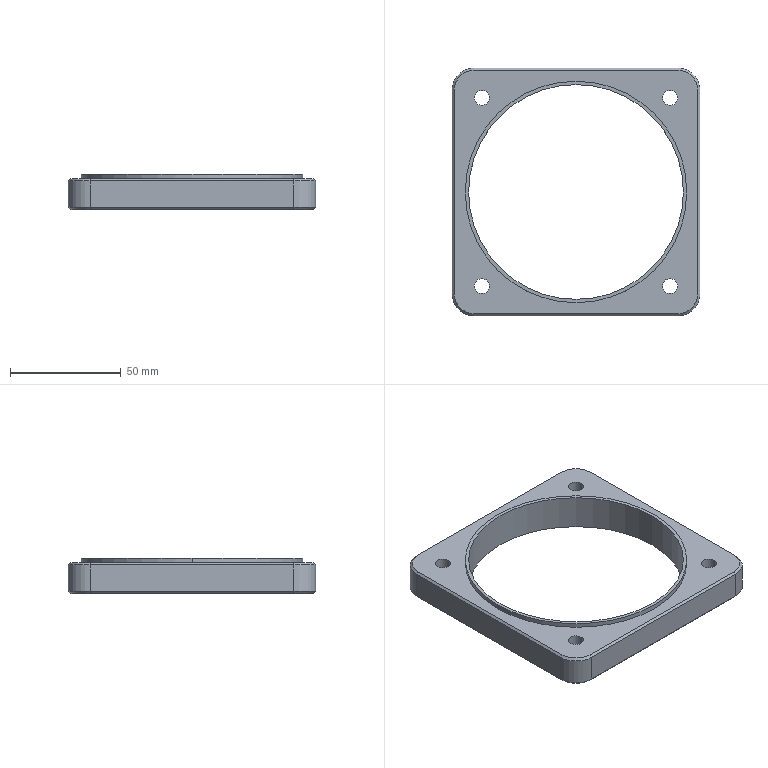Part | SolidWorks | features ICE 2, Chamfer 1, Extrusion 1, HoleWzd 1 | 1 solid | 39 faces | box 112 x 112 x 16 mm | volume 69423 mm3 | cylinder 16 | plane 15 | cone 8 | commonest cylinder face diameters 6.8 x8 20 x4 97 x2 100 x2
STEP:
#1=CARTESIAN_POINT('',(50.,0.,14.));
#2=VERTEX_POINT('',#1);
#3=CARTESIAN_POINT('',(-50.,0.,14.));
#4=VERTEX_POINT('',#3);
#5=CARTESIAN_POINT('',(0.,0.,14.));
#6=DIRECTION('',(0.,0.,1.));
#7=DIRECTION('',(1.,0.,0.));
#8=AXIS2_PLACEMENT_3D('',#5,#6,#7);
#9=CIRCLE('',#8,50.);
#10=EDGE_CURVE('',#2,#4,#9,.T.);
#11=ORIENTED_EDGE('',*,*,#10,.T.);
#12=CARTESIAN_POINT('',(-50.,0.,16.));
#13=VERTEX_POINT('',#12);
#14=CARTESIAN_POINT('',(-50.,0.,14.));
#15=DIRECTION('',(0.,0.,1.));
#16=VECTOR('',#15,1000.);
#17=LINE('',#14,#16);
#18=EDGE_CURVE('',#4,#13,#17,.T.);
#19=ORIENTED_EDGE('',*,*,#18,.T.);
#20=CARTESIAN_POINT('',(50.,0.,16.));
#21=VERTEX_POINT('',#20);
#22=CARTESIAN_POINT('',(0.,0.,16.));
#23=DIRECTION('',(0.,0.,1.));
#24=DIRECTION('',(1.,0.,0.));
#25=AXIS2_PLACEMENT_3D('',#22,#23,#24);
#26=CIRCLE('',#25,50.);
#27=EDGE_CURVE('',#21,#13,#26,.T.);
#28=ORIENTED_EDGE('',*,*,#27,.F.);
#29=CARTESIAN_POINT('',(50.,0.,14.));
#30=DIRECTION('',(0.,0.,1.));
#31=VECTOR('',#30,1000.);
#32=LINE('',#29,#31);
#33=EDGE_CURVE('',#2,#21,#32,.T.);
#34=ORIENTED_EDGE('',*,*,#33,.F.);
#35=EDGE_LOOP('',(#11,#19,#28,#34));
#36=FACE_OUTER_BOUND('',#35,.T.);
#37=CARTESIAN_POINT('',(0.,0.,14.));
#38=DIRECTION('',(0.,0.,1.));
#39=DIRECTION('',(1.,0.,0.));
#40=AXIS2_PLACEMENT_3D('',#37,#38,#39);
#41=CYLINDRICAL_SURFACE('',#40,50.);
#42=ADVANCED_FACE('',(#36),#41,.T.);
#43=CARTESIAN_POINT('',(-48.5,0.,16.));
#44=VERTEX_POINT('',#43);
#45=CARTESIAN_POINT('',(48.5,0.,16.));
#46=VERTEX_POINT('',#45);
#47=CARTESIAN_POINT('',(0.,0.,16.));
#48=DIRECTION('',(0.,0.,1.));
#49=DIRECTION('',(1.,0.,0.));
#50=AXIS2_PLACEMENT_3D('',#47,#48,#49);
#51=CIRCLE('',#50,48.5);
#52=EDGE_CURVE('',#44,#46,#51,.T.);
#53=ORIENTED_EDGE('',*,*,#52,.T.);
#54=CARTESIAN_POINT('',(48.5,0.,0.));
#55=VERTEX_POINT('',#54);
#56=CARTESIAN_POINT('',(48.5,0.,16.));
#57=DIRECTION('',(0.,0.,-1.));
#58=VECTOR('',#57,1000.);
#59=LINE('',#56,#58);
#60=EDGE_CURVE('',#46,#55,#59,.T.);
#61=ORIENTED_EDGE('',*,*,#60,.T.);
#62=CARTESIAN_POINT('',(-48.5,0.,0.));
#63=VERTEX_POINT('',#62);
#64=CARTESIAN_POINT('',(0.,0.,0.));
#65=DIRECTION('',(0.,0.,1.));
#66=DIRECTION('',(1.,0.,0.));
#67=AXIS2_PLACEMENT_3D('',#64,#65,#66);
#68=CIRCLE('',#67,48.5);
#69=EDGE_CURVE('',#63,#55,#68,.T.);
#70=ORIENTED_EDGE('',*,*,#69,.F.);
#71=CARTESIAN_POINT('',(-48.5,0.,16.));
#72=DIRECTION('',(0.,0.,-1.));
#73=VECTOR('',#72,1000.);
#74=LINE('',#71,#73);
#75=EDGE_CURVE('',#44,#63,#74,.T.);
#76=ORIENTED_EDGE('',*,*,#75,.F.);
#77=EDGE_LOOP('',(#53,#61,#70,#76));
#78=FACE_OUTER_BOUND('',#77,.T.);
#79=CARTESIAN_POINT('',(0.,0.,16.));
#80=DIRECTION('',(0.,0.,-1.));
#81=DIRECTION('',(-1.,0.,0.));
#82=AXIS2_PLACEMENT_3D('',#79,#80,#81);
#83=CYLINDRICAL_SURFACE('',#82,48.5);
#84=ADVANCED_FACE('',(#78),#83,.F.);
#85=CARTESIAN_POINT('',(-45.9,42.5,0.));
#86=VERTEX_POINT('',#85);
#87=CARTESIAN_POINT('',(-39.1,42.5,0.));
#88=VERTEX_POINT('',#87);
#89=CARTESIAN_POINT('',(-42.5,42.5,0.));
#90=DIRECTION('',(0.,0.,1.));
#91=DIRECTION('',(1.,0.,0.));
#92=AXIS2_PLACEMENT_3D('',#89,#90,#91);
#93=CIRCLE('',#92,3.4);
#94=EDGE_CURVE('',#86,#88,#93,.T.);
#95=ORIENTED_EDGE('',*,*,#94,.F.);
#96=CARTESIAN_POINT('',(-45.9,42.5,14.));
#97=VERTEX_POINT('',#96);
#98=CARTESIAN_POINT('',(-45.9,42.5,16.));
#99=DIRECTION('',(0.,0.,1.));
#100=VECTOR('',#99,1000.);
#101=LINE('',#98,#100);
#102=EDGE_CURVE('',#86,#97,#101,.T.);
#103=ORIENTED_EDGE('',*,*,#102,.T.);
#104=CARTESIAN_POINT('',(-39.1,42.5,14.));
#105=VERTEX_POINT('',#104);
#106=CARTESIAN_POINT('',(-42.5,42.5,14.));
#107=DIRECTION('',(0.,0.,-1.));
#108=DIRECTION('',(1.,0.,0.));
#109=AXIS2_PLACEMENT_3D('',#106,#107,#108);
#110=CIRCLE('',#109,3.4);
#111=EDGE_CURVE('',#105,#97,#110,.T.);
#112=ORIENTED_EDGE('',*,*,#111,.F.);
#113=CARTESIAN_POINT('',(-39.1,42.5,16.));
#114=DIRECTION('',(0.,0.,1.));
#115=VECTOR('',#114,1000.);
#116=LINE('',#113,#115);
#117=EDGE_CURVE('',#88,#105,#116,.T.);
#118=ORIENTED_EDGE('',*,*,#117,.F.);
#119=EDGE_LOOP('',(#95,#103,#112,#118));
#120=FACE_OUTER_BOUND('',#119,.T.);
#121=CARTESIAN_POINT('',(-42.5,42.5,16.));
#122=DIRECTION('',(0.,0.,1.));
#123=DIRECTION('',(1.,0.,0.));
#124=AXIS2_PLACEMENT_3D('',#121,#122,#123);
#125=CYLINDRICAL_SURFACE('',#124,3.4);
#126=ADVANCED_FACE('',(#120),#125,.F.);
#127=CARTESIAN_POINT('',(39.1,42.5,0.));
#128=VERTEX_POINT('',#127);
#129=CARTESIAN_POINT('',(45.9,42.5,0.));
#130=VERTEX_POINT('',#129);
#131=CARTESIAN_POINT('',(42.5,42.5,0.));
#132=DIRECTION('',(0.,0.,1.));
#133=DIRECTION('',(1.,0.,0.));
#134=AXIS2_PLACEMENT_3D('',#131,#132,#133);
#135=CIRCLE('',#134,3.4);
#136=EDGE_CURVE('',#128,#130,#135,.T.);
#137=ORIENTED_EDGE('',*,*,#136,.F.);
#138=CARTESIAN_POINT('',(39.1,42.5,14.));
#139=VERTEX_POINT('',#138);
#140=CARTESIAN_POINT('',(39.1,42.5,16.));
#141=DIRECTION('',(0.,0.,1.));
#142=VECTOR('',#141,1000.);
#143=LINE('',#140,#142);
#144=EDGE_CURVE('',#128,#139,#143,.T.);
#145=ORIENTED_EDGE('',*,*,#144,.T.);
#146=CARTESIAN_POINT('',(45.9,42.5,14.));
#147=VERTEX_POINT('',#146);
#148=CARTESIAN_POINT('',(42.5,42.5,14.));
#149=DIRECTION('',(0.,0.,-1.));
#150=DIRECTION('',(1.,0.,0.));
#151=AXIS2_PLACEMENT_3D('',#148,#149,#150);
#152=CIRCLE('',#151,3.4);
#153=EDGE_CURVE('',#147,#139,#152,.T.);
#154=ORIENTED_EDGE('',*,*,#153,.F.);
#155=CARTESIAN_POINT('',(45.9,42.5,16.));
#156=DIRECTION('',(0.,0.,1.));
#157=VECTOR('',#156,1000.);
#158=LINE('',#155,#157);
#159=EDGE_CURVE('',#130,#147,#158,.T.);
#160=ORIENTED_EDGE('',*,*,#159,.F.);
#161=EDGE_LOOP('',(#137,#145,#154,#160));
#162=FACE_OUTER_BOUND('',#161,.T.);
#163=CARTESIAN_POINT('',(42.5,42.5,16.));
#164=DIRECTION('',(0.,0.,1.));
#165=DIRECTION('',(1.,0.,0.));
#166=AXIS2_PLACEMENT_3D('',#163,#164,#165);
#167=CYLINDRICAL_SURFACE('',#166,3.4);
#168=ADVANCED_FACE('',(#162),#167,.F.);
#169=CARTESIAN_POINT('',(39.1,-42.5,0.));
#170=VERTEX_POINT('',#169);
#171=CARTESIAN_POINT('',(45.9,-42.5,0.));
#172=VERTEX_POINT('',#171);
#173=CARTESIAN_POINT('',(42.5,-42.5,0.));
#174=DIRECTION('',(0.,0.,1.));
#175=DIRECTION('',(1.,0.,0.));
#176=AXIS2_PLACEMENT_3D('',#173,#174,#175);
#177=CIRCLE('',#176,3.4);
#178=EDGE_CURVE('',#170,#172,#177,.T.);
#179=ORIENTED_EDGE('',*,*,#178,.F.);
#180=CARTESIAN_POINT('',(39.1,-42.5,14.));
#181=VERTEX_POINT('',#180);
#182=CARTESIAN_POINT('',(39.1,-42.5,16.));
#183=DIRECTION('',(0.,0.,1.));
#184=VECTOR('',#183,1000.);
#185=LINE('',#182,#184);
#186=EDGE_CURVE('',#170,#181,#185,.T.);
#187=ORIENTED_EDGE('',*,*,#186,.T.);
#188=CARTESIAN_POINT('',(45.9,-42.5,14.));
#189=VERTEX_POINT('',#188);
#190=CARTESIAN_POINT('',(42.5,-42.5,14.));
#191=DIRECTION('',(0.,0.,-1.));
#192=DIRECTION('',(1.,0.,0.));
#193=AXIS2_PLACEMENT_3D('',#190,#191,#192);
#194=CIRCLE('',#193,3.4);
#195=EDGE_CURVE('',#189,#181,#194,.T.);
#196=ORIENTED_EDGE('',*,*,#195,.F.);
#197=CARTESIAN_POINT('',(45.9,-42.5,16.));
#198=DIRECTION('',(0.,0.,1.));
#199=VECTOR('',#198,1000.);
#200=LINE('',#197,#199);
#201=EDGE_CURVE('',#172,#189,#200,.T.);
#202=ORIENTED_EDGE('',*,*,#201,.F.);
#203=EDGE_LOOP('',(#179,#187,#196,#202));
#204=FACE_OUTER_BOUND('',#203,.T.);
#205=CARTESIAN_POINT('',(42.5,-42.5,16.));
#206=DIRECTION('',(0.,0.,1.));
#207=DIRECTION('',(1.,0.,0.));
#208=AXIS2_PLACEMENT_3D('',#205,#206,#207);
#209=CYLINDRICAL_SURFACE('',#208,3.4);
#210=ADVANCED_FACE('',(#204),#209,.F.);
#211=CARTESIAN_POINT('',(-45.9,-42.5,0.));
#212=VERTEX_POINT('',#211);
#213=CARTESIAN_POINT('',(-39.1,-42.5,0.));
#214=VERTEX_POINT('',#213);
#215=CARTESIAN_POINT('',(-42.5,-42.5,0.));
#216=DIRECTION('',(0.,0.,1.));
#217=DIRECTION('',(1.,0.,0.));
#218=AXIS2_PLACEMENT_3D('',#215,#216,#217);
#219=CIRCLE('',#218,3.4);
#220=EDGE_CURVE('',#212,#214,#219,.T.);
#221=ORIENTED_EDGE('',*,*,#220,.F.);
#222=CARTESIAN_POINT('',(-45.9,-42.5,14.));
#223=VERTEX_POINT('',#222);
#224=CARTESIAN_POINT('',(-45.9,-42.5,16.));
#225=DIRECTION('',(0.,0.,1.));
#226=VECTOR('',#225,1000.);
#227=LINE('',#224,#226);
#228=EDGE_CURVE('',#212,#223,#227,.T.);
#229=ORIENTED_EDGE('',*,*,#228,.T.);
#230=CARTESIAN_POINT('',(-39.1,-42.5,14.));
#231=VERTEX_POINT('',#230);
#232=CARTESIAN_POINT('',(-42.5,-42.5,14.));
#233=DIRECTION('',(0.,0.,-1.));
#234=DIRECTION('',(1.,0.,0.));
#235=AXIS2_PLACEMENT_3D('',#232,#233,#234);
#236=CIRCLE('',#235,3.4);
#237=EDGE_CURVE('',#231,#223,#236,.T.);
#238=ORIENTED_EDGE('',*,*,#237,.F.);
#239=CARTESIAN_POINT('',(-39.1,-42.5,16.));
#240=DIRECTION('',(0.,0.,1.));
#241=VECTOR('',#240,1000.);
#242=LINE('',#239,#241);
#243=EDGE_CURVE('',#214,#231,#242,.T.);
#244=ORIENTED_EDGE('',*,*,#243,.F.);
#245=EDGE_LOOP('',(#221,#229,#238,#244));
#246=FACE_OUTER_BOUND('',#245,.T.);
#247=CARTESIAN_POINT('',(-42.5,-42.5,16.));
#248=DIRECTION('',(0.,0.,1.));
#249=DIRECTION('',(1.,0.,0.));
#250=AXIS2_PLACEMENT_3D('',#247,#248,#249);
#251=CYLINDRICAL_SURFACE('',#250,3.4);
#252=ADVANCED_FACE('',(#246),#251,.F.);
#253=ORIENTED_EDGE('',*,*,#52,.F.);
#254=CARTESIAN_POINT('',(0.,0.,16.));
#255=DIRECTION('',(0.,0.,1.));
#256=DIRECTION('',(1.,0.,0.));
#257=AXIS2_PLACEMENT_3D('',#254,#255,#256);
#258=CIRCLE('',#257,48.5);
#259=EDGE_CURVE('',#46,#44,#258,.T.);
#260=ORIENTED_EDGE('',*,*,#259,.F.);
#261=EDGE_LOOP('',(#253,#260));
#262=FACE_BOUND('',#261,.T.);
#263=ORIENTED_EDGE('',*,*,#27,.T.);
#264=CARTESIAN_POINT('',(0.,0.,16.));
#265=DIRECTION('',(0.,0.,1.));
#266=DIRECTION('',(1.,0.,0.));
#267=AXIS2_PLACEMENT_3D('',#264,#265,#266);
#268=CIRCLE('',#267,50.);
#269=EDGE_CURVE('',#13,#21,#268,.T.);
#270=ORIENTED_EDGE('',*,*,#269,.T.);
#271=EDGE_LOOP('',(#263,#270));
#272=FACE_OUTER_BOUND('',#271,.T.);
#273=CARTESIAN_POINT('',(-46.,-46.,16.));
#274=DIRECTION('',(0.,0.,1.));
#275=DIRECTION('',(1.,0.,0.));
#276=AXIS2_PLACEMENT_3D('',#273,#274,#275);
#277=PLANE('',#276);
#278=ADVANCED_FACE('',(#262,#272),#277,.T.);
#279=CARTESIAN_POINT('',(-46.,-56.,13.));
#280=VERTEX_POINT('',#279);
#281=CARTESIAN_POINT('',(-46.,-56.,1.));
#282=VERTEX_POINT('',#281);
#283=CARTESIAN_POINT('',(-46.,-56.,16.));
#284=DIRECTION('',(0.,0.,-1.));
#285=VECTOR('',#284,1000.);
#286=LINE('',#283,#285);
#287=EDGE_CURVE('',#280,#282,#286,.T.);
#288=ORIENTED_EDGE('',*,*,#287,.F.);
#289=CARTESIAN_POINT('',(-56.,-46.,13.));
#290=VERTEX_POINT('',#289);
#291=CARTESIAN_POINT('',(-46.,-46.,13.));
#292=DIRECTION('',(0.,0.,-1.));
#293=DIRECTION('',(1.,0.,0.));
#294=AXIS2_PLACEMENT_3D('',#291,#292,#293);
#295=CIRCLE('',#294,10.);
#296=EDGE_CURVE('',#280,#290,#295,.T.);
#297=ORIENTED_EDGE('',*,*,#296,.T.);
#298=CARTESIAN_POINT('',(-56.,-46.,1.));
#299=VERTEX_POINT('',#298);
#300=CARTESIAN_POINT('',(-56.,-46.,16.));
#301=DIRECTION('',(0.,0.,-1.));
#302=VECTOR('',#301,1000.);
#303=LINE('',#300,#302);
#304=EDGE_CURVE('',#290,#299,#303,.T.);
#305=ORIENTED_EDGE('',*,*,#304,.T.);
#306=CARTESIAN_POINT('',(-46.,-46.,1.));
#307=DIRECTION('',(0.,0.,1.));
#308=DIRECTION('',(1.,0.,0.));
#309=AXIS2_PLACEMENT_3D('',#306,#307,#308);
#310=CIRCLE('',#309,10.);
#311=EDGE_CURVE('',#299,#282,#310,.T.);
#312=ORIENTED_EDGE('',*,*,#311,.T.);
#313=EDGE_LOOP('',(#288,#297,#305,#312));
#314=FACE_OUTER_BOUND('',#313,.T.);
#315=CARTESIAN_POINT('',(-46.,-46.,16.));
#316=DIRECTION('',(0.,0.,-1.));
#317=DIRECTION('',(-1.,0.,0.));
#318=AXIS2_PLACEMENT_3D('',#315,#316,#317);
#319=CYLINDRICAL_SURFACE('',#318,10.);
#320=ADVANCED_FACE('',(#314),#319,.T.);
#321=CARTESIAN_POINT('',(46.,-56.,13.));
#322=VERTEX_POINT('',#321);
#323=CARTESIAN_POINT('',(46.,-56.,1.));
#324=VERTEX_POINT('',#323);
#325=CARTESIAN_POINT('',(46.,-56.,16.));
#326=DIRECTION('',(0.,0.,-1.));
#327=VECTOR('',#326,1000.);
#328=LINE('',#325,#327);
#329=EDGE_CURVE('',#322,#324,#328,.T.);
#330=ORIENTED_EDGE('',*,*,#329,.F.);
#331=CARTESIAN_POINT('',(-46.,-56.,13.));
#332=DIRECTION('',(-1.,0.,0.));
#333=VECTOR('',#332,1000.);
#334=LINE('',#331,#333);
#335=EDGE_CURVE('',#322,#280,#334,.T.);
#336=ORIENTED_EDGE('',*,*,#335,.T.);
#337=ORIENTED_EDGE('',*,*,#287,.T.);
#338=CARTESIAN_POINT('',(-46.,-56.,1.));
#339=DIRECTION('',(1.,0.,0.));
#340=VECTOR('',#339,1000.);
#341=LINE('',#338,#340);
#342=EDGE_CURVE('',#282,#324,#341,.T.);
#343=ORIENTED_EDGE('',*,*,#342,.T.);
#344=EDGE_LOOP('',(#330,#336,#337,#343));
#345=FACE_OUTER_BOUND('',#344,.T.);
#346=CARTESIAN_POINT('',(-46.,-56.,16.));
#347=DIRECTION('',(0.,1.,0.));
#348=DIRECTION('',(0.,0.,1.));
#349=AXIS2_PLACEMENT_3D('',#346,#347,#348);
#350=PLANE('',#349);
#351=ADVANCED_FACE('',(#345),#350,.F.);
#352=CARTESIAN_POINT('',(56.,-46.,13.));
#353=VERTEX_POINT('',#352);
#354=CARTESIAN_POINT('',(56.,-46.,1.));
#355=VERTEX_POINT('',#354);
#356=CARTESIAN_POINT('',(56.,-46.,16.));
#357=DIRECTION('',(0.,0.,-1.));
#358=VECTOR('',#357,1000.);
#359=LINE('',#356,#358);
#360=EDGE_CURVE('',#353,#355,#359,.T.);
#361=ORIENTED_EDGE('',*,*,#360,.F.);
#362=CARTESIAN_POINT('',(46.,-46.,13.));
#363=DIRECTION('',(0.,0.,-1.));
#364=DIRECTION('',(1.,0.,0.));
#365=AXIS2_PLACEMENT_3D('',#362,#363,#364);
#366=CIRCLE('',#365,10.);
#367=EDGE_CURVE('',#353,#322,#366,.T.);
#368=ORIENTED_EDGE('',*,*,#367,.T.);
#369=ORIENTED_EDGE('',*,*,#329,.T.);
#370=CARTESIAN_POINT('',(46.,-46.,1.));
#371=DIRECTION('',(0.,0.,1.));
#372=DIRECTION('',(1.,0.,0.));
#373=AXIS2_PLACEMENT_3D('',#370,#371,#372);
#374=CIRCLE('',#373,10.);
#375=EDGE_CURVE('',#324,#355,#374,.T.);
#376=ORIENTED_EDGE('',*,*,#375,.T.);
#377=EDGE_LOOP('',(#361,#368,#369,#376));
#378=FACE_OUTER_BOUND('',#377,.T.);
#379=CARTESIAN_POINT('',(46.,-46.,16.));
#380=DIRECTION('',(0.,0.,-1.));
#381=DIRECTION('',(-1.,0.,0.));
#382=AXIS2_PLACEMENT_3D('',#379,#380,#381);
#383=CYLINDRICAL_SURFACE('',#382,10.);
#384=ADVANCED_FACE('',(#378),#383,.T.);
#385=CARTESIAN_POINT('',(56.,46.,13.));
#386=VERTEX_POINT('',#385);
#387=CARTESIAN_POINT('',(56.,46.,1.));
#388=VERTEX_POINT('',#387);
#389=CARTESIAN_POINT('',(56.,46.,16.));
#390=DIRECTION('',(0.,0.,-1.));
#391=VECTOR('',#390,1000.);
#392=LINE('',#389,#391);
#393=EDGE_CURVE('',#386,#388,#392,.T.);
#394=ORIENTED_EDGE('',*,*,#393,.F.);
#395=CARTESIAN_POINT('',(56.,-46.,13.));
#396=DIRECTION('',(0.,-1.,0.));
#397=VECTOR('',#396,1000.);
#398=LINE('',#395,#397);
#399=EDGE_CURVE('',#386,#353,#398,.T.);
#400=ORIENTED_EDGE('',*,*,#399,.T.);
#401=ORIENTED_EDGE('',*,*,#360,.T.);
#402=CARTESIAN_POINT('',(56.,46.,1.));
#403=DIRECTION('',(0.,1.,0.));
#404=VECTOR('',#403,1000.);
#405=LINE('',#402,#404);
#406=EDGE_CURVE('',#355,#388,#405,.T.);
#407=ORIENTED_EDGE('',*,*,#406,.T.);
#408=EDGE_LOOP('',(#394,#400,#401,#407));
#409=FACE_OUTER_BOUND('',#408,.T.);
#410=CARTESIAN_POINT('',(56.,46.,16.));
#411=DIRECTION('',(-1.,0.,0.));
#412=DIRECTION('',(0.,-1.,0.));
#413=AXIS2_PLACEMENT_3D('',#410,#411,#412);
#414=PLANE('',#413);
#415=ADVANCED_FACE('',(#409),#414,.F.);
#416=CARTESIAN_POINT('',(46.,56.,13.));
#417=VERTEX_POINT('',#416);
#418=CARTESIAN_POINT('',(46.,56.,1.));
#419=VERTEX_POINT('',#418);
#420=CARTESIAN_POINT('',(46.,56.,16.));
#421=DIRECTION('',(0.,0.,-1.));
#422=VECTOR('',#421,1000.);
#423=LINE('',#420,#422);
#424=EDGE_CURVE('',#417,#419,#423,.T.);
#425=ORIENTED_EDGE('',*,*,#424,.F.);
#426=CARTESIAN_POINT('',(46.,46.,13.));
#427=DIRECTION('',(0.,0.,-1.));
#428=DIRECTION('',(1.,0.,0.));
#429=AXIS2_PLACEMENT_3D('',#426,#427,#428);
#430=CIRCLE('',#429,10.);
#431=EDGE_CURVE('',#417,#386,#430,.T.);
#432=ORIENTED_EDGE('',*,*,#431,.T.);
#433=ORIENTED_EDGE('',*,*,#393,.T.);
#434=CARTESIAN_POINT('',(46.,46.,1.));
#435=DIRECTION('',(0.,0.,1.));
#436=DIRECTION('',(1.,0.,0.));
#437=AXIS2_PLACEMENT_3D('',#434,#435,#436);
#438=CIRCLE('',#437,10.);
#439=EDGE_CURVE('',#388,#419,#438,.T.);
#440=ORIENTED_EDGE('',*,*,#439,.T.);
#441=EDGE_LOOP('',(#425,#432,#433,#440));
#442=FACE_OUTER_BOUND('',#441,.T.);
#443=CARTESIAN_POINT('',(46.,46.,16.));
#444=DIRECTION('',(0.,0.,-1.));
#445=DIRECTION('',(-1.,0.,0.));
#446=AXIS2_PLACEMENT_3D('',#443,#444,#445);
#447=CYLINDRICAL_SURFACE('',#446,10.);
#448=ADVANCED_FACE('',(#442),#447,.T.);
#449=CARTESIAN_POINT('',(-46.,56.,13.));
#450=VERTEX_POINT('',#449);
#451=CARTESIAN_POINT('',(-46.,56.,1.));
#452=VERTEX_POINT('',#451);
#453=CARTESIAN_POINT('',(-46.,56.,16.));
#454=DIRECTION('',(0.,0.,-1.));
#455=VECTOR('',#454,1000.);
#456=LINE('',#453,#455);
#457=EDGE_CURVE('',#450,#452,#456,.T.);
#458=ORIENTED_EDGE('',*,*,#457,.F.);
#459=CARTESIAN_POINT('',(46.,56.,13.));
#460=DIRECTION('',(1.,0.,0.));
#461=VECTOR('',#460,1000.);
#462=LINE('',#459,#461);
#463=EDGE_CURVE('',#450,#417,#462,.T.);
#464=ORIENTED_EDGE('',*,*,#463,.T.);
#465=ORIENTED_EDGE('',*,*,#424,.T.);
#466=CARTESIAN_POINT('',(-46.,56.,1.));
#467=DIRECTION('',(-1.,0.,0.));
#468=VECTOR('',#467,1000.);
#469=LINE('',#466,#468);
#470=EDGE_CURVE('',#419,#452,#469,.T.);
#471=ORIENTED_EDGE('',*,*,#470,.T.);
#472=EDGE_LOOP('',(#458,#464,#465,#471));
#473=FACE_OUTER_BOUND('',#472,.T.);
#474=CARTESIAN_POINT('',(-46.,56.,16.));
#475=DIRECTION('',(0.,-1.,0.));
#476=DIRECTION('',(0.,0.,-1.));
#477=AXIS2_PLACEMENT_3D('',#474,#475,#476);
#478=PLANE('',#477);
#479=ADVANCED_FACE('',(#473),#478,.F.);
#480=CARTESIAN_POINT('',(-56.,46.,13.));
#481=VERTEX_POINT('',#480);
#482=CARTESIAN_POINT('',(-56.,46.,1.));
#483=VERTEX_POINT('',#482);
#484=CARTESIAN_POINT('',(-56.,46.,16.));
#485=DIRECTION('',(0.,0.,-1.));
#486=VECTOR('',#485,1000.);
#487=LINE('',#484,#486);
#488=EDGE_CURVE('',#481,#483,#487,.T.);
#489=ORIENTED_EDGE('',*,*,#488,.F.);
#490=CARTESIAN_POINT('',(-46.,46.,13.));
#491=DIRECTION('',(0.,0.,-1.));
#492=DIRECTION('',(1.,0.,0.));
#493=AXIS2_PLACEMENT_3D('',#490,#491,#492);
#494=CIRCLE('',#493,10.);
#495=EDGE_CURVE('',#481,#450,#494,.T.);
#496=ORIENTED_EDGE('',*,*,#495,.T.);
#497=ORIENTED_EDGE('',*,*,#457,.T.);
#498=CARTESIAN_POINT('',(-46.,46.,1.));
#499=DIRECTION('',(0.,0.,1.));
#500=DIRECTION('',(1.,0.,0.));
#501=AXIS2_PLACEMENT_3D('',#498,#499,#500);
#502=CIRCLE('',#501,10.);
#503=EDGE_CURVE('',#452,#483,#502,.T.);
#504=ORIENTED_EDGE('',*,*,#503,.T.);
#505=EDGE_LOOP('',(#489,#496,#497,#504));
#506=FACE_OUTER_BOUND('',#505,.T.);
#507=CARTESIAN_POINT('',(-46.,46.,16.));
#508=DIRECTION('',(0.,0.,-1.));
#509=DIRECTION('',(-1.,0.,0.));
#510=AXIS2_PLACEMENT_3D('',#507,#508,#509);
#511=CYLINDRICAL_SURFACE('',#510,10.);
#512=ADVANCED_FACE('',(#506),#511,.T.);
#513=ORIENTED_EDGE('',*,*,#304,.F.);
#514=CARTESIAN_POINT('',(-56.,46.,13.));
#515=DIRECTION('',(0.,1.,0.));
#516=VECTOR('',#515,1000.);
#517=LINE('',#514,#516);
#518=EDGE_CURVE('',#290,#481,#517,.T.);
#519=ORIENTED_EDGE('',*,*,#518,.T.);
#520=ORIENTED_EDGE('',*,*,#488,.T.);
#521=CARTESIAN_POINT('',(-56.,46.,1.));
#522=DIRECTION('',(0.,-1.,0.));
#523=VECTOR('',#522,1000.);
#524=LINE('',#521,#523);
#525=EDGE_CURVE('',#483,#299,#524,.T.);
#526=ORIENTED_EDGE('',*,*,#525,.T.);
#527=EDGE_LOOP('',(#513,#519,#520,#526));
#528=FACE_OUTER_BOUND('',#527,.T.);
#529=CARTESIAN_POINT('',(-56.,46.,16.));
#530=DIRECTION('',(1.,0.,0.));
#531=DIRECTION('',(0.,1.,0.));
#532=AXIS2_PLACEMENT_3D('',#529,#530,#531);
#533=PLANE('',#532);
#534=ADVANCED_FACE('',(#528),#533,.F.);
#535=ORIENTED_EDGE('',*,*,#228,.F.);
#536=CARTESIAN_POINT('',(-42.5,-42.5,0.));
#537=DIRECTION('',(0.,0.,1.));
#538=DIRECTION('',(1.,0.,0.));
#539=AXIS2_PLACEMENT_3D('',#536,#537,#538);
#540=CIRCLE('',#539,3.4);
#541=EDGE_CURVE('',#214,#212,#540,.T.);
#542=ORIENTED_EDGE('',*,*,#541,.F.);
#543=ORIENTED_EDGE('',*,*,#243,.T.);
#544=CARTESIAN_POINT('',(-42.5,-42.5,14.));
#545=DIRECTION('',(0.,0.,-1.));
#546=DIRECTION('',(1.,0.,0.));
#547=AXIS2_PLACEMENT_3D('',#544,#545,#546);
#548=CIRCLE('',#547,3.4);
#549=EDGE_CURVE('',#223,#231,#548,.T.);
#550=ORIENTED_EDGE('',*,*,#549,.F.);
#551=EDGE_LOOP('',(#535,#542,#543,#550));
#552=FACE_OUTER_BOUND('',#551,.T.);
#553=CARTESIAN_POINT('',(-42.5,-42.5,16.));
#554=DIRECTION('',(0.,0.,1.));
#555=DIRECTION('',(1.,0.,0.));
#556=AXIS2_PLACEMENT_3D('',#553,#554,#555);
#557=CYLINDRICAL_SURFACE('',#556,3.4);
#558=ADVANCED_FACE('',(#552),#557,.F.);
#559=ORIENTED_EDGE('',*,*,#186,.F.);
#560=CARTESIAN_POINT('',(42.5,-42.5,0.));
#561=DIRECTION('',(0.,0.,1.));
#562=DIRECTION('',(1.,0.,0.));
#563=AXIS2_PLACEMENT_3D('',#560,#561,#562);
#564=CIRCLE('',#563,3.4);
#565=EDGE_CURVE('',#172,#170,#564,.T.);
#566=ORIENTED_EDGE('',*,*,#565,.F.);
#567=ORIENTED_EDGE('',*,*,#201,.T.);
#568=CARTESIAN_POINT('',(42.5,-42.5,14.));
#569=DIRECTION('',(0.,0.,-1.));
#570=DIRECTION('',(1.,0.,0.));
#571=AXIS2_PLACEMENT_3D('',#568,#569,#570);
#572=CIRCLE('',#571,3.4);
#573=EDGE_CURVE('',#181,#189,#572,.T.);
#574=ORIENTED_EDGE('',*,*,#573,.F.);
#575=EDGE_LOOP('',(#559,#566,#567,#574));
#576=FACE_OUTER_BOUND('',#575,.T.);
#577=CARTESIAN_POINT('',(42.5,-42.5,16.));
#578=DIRECTION('',(0.,0.,1.));
#579=DIRECTION('',(1.,0.,0.));
#580=AXIS2_PLACEMENT_3D('',#577,#578,#579);
#581=CYLINDRICAL_SURFACE('',#580,3.4);
#582=ADVANCED_FACE('',(#576),#581,.F.);
#583=ORIENTED_EDGE('',*,*,#144,.F.);
#584=CARTESIAN_POINT('',(42.5,42.5,0.));
#585=DIRECTION('',(0.,0.,1.));
#586=DIRECTION('',(1.,0.,0.));
#587=AXIS2_PLACEMENT_3D('',#584,#585,#586);
#588=CIRCLE('',#587,3.4);
#589=EDGE_CURVE('',#130,#128,#588,.T.);
#590=ORIENTED_EDGE('',*,*,#589,.F.);
#591=ORIENTED_EDGE('',*,*,#159,.T.);
#592=CARTESIAN_POINT('',(42.5,42.5,14.));
#593=DIRECTION('',(0.,0.,-1.));
#594=DIRECTION('',(1.,0.,0.));
#595=AXIS2_PLACEMENT_3D('',#592,#593,#594);
#596=CIRCLE('',#595,3.4);
#597=EDGE_CURVE('',#139,#147,#596,.T.);
#598=ORIENTED_EDGE('',*,*,#597,.F.);
#599=EDGE_LOOP('',(#583,#590,#591,#598));
#600=FACE_OUTER_BOUND('',#599,.T.);
#601=CARTESIAN_POINT('',(42.5,42.5,16.));
#602=DIRECTION('',(0.,0.,1.));
#603=DIRECTION('',(1.,0.,0.));
#604=AXIS2_PLACEMENT_3D('',#601,#602,#603);
#605=CYLINDRICAL_SURFACE('',#604,3.4);
#606=ADVANCED_FACE('',(#600),#605,.F.);
#607=ORIENTED_EDGE('',*,*,#102,.F.);
#608=CARTESIAN_POINT('',(-42.5,42.5,0.));
#609=DIRECTION('',(0.,0.,1.));
#610=DIRECTION('',(1.,0.,0.));
#611=AXIS2_PLACEMENT_3D('',#608,#609,#610);
#612=CIRCLE('',#611,3.4);
#613=EDGE_CURVE('',#88,#86,#612,.T.);
#614=ORIENTED_EDGE('',*,*,#613,.F.);
#615=ORIENTED_EDGE('',*,*,#117,.T.);
#616=CARTESIAN_POINT('',(-42.5,42.5,14.));
#617=DIRECTION('',(0.,0.,-1.));
#618=DIRECTION('',(1.,0.,0.));
#619=AXIS2_PLACEMENT_3D('',#616,#617,#618);
#620=CIRCLE('',#619,3.4);
#621=EDGE_CURVE('',#97,#105,#620,.T.);
#622=ORIENTED_EDGE('',*,*,#621,.F.);
#623=EDGE_LOOP('',(#607,#614,#615,#622));
#624=FACE_OUTER_BOUND('',#623,.T.);
#625=CARTESIAN_POINT('',(-42.5,42.5,16.));
#626=DIRECTION('',(0.,0.,1.));
#627=DIRECTION('',(1.,0.,0.));
#628=AXIS2_PLACEMENT_3D('',#625,#626,#627);
#629=CYLINDRICAL_SURFACE('',#628,3.4);
#630=ADVANCED_FACE('',(#624),#629,.F.);
#631=CARTESIAN_POINT('',(46.,55.,0.));
#632=VERTEX_POINT('',#631);
#633=CARTESIAN_POINT('',(55.,46.,0.));
#634=VERTEX_POINT('',#633);
#635=CARTESIAN_POINT('',(46.,46.,0.));
#636=DIRECTION('',(0.,0.,-1.));
#637=DIRECTION('',(1.,0.,0.));
#638=AXIS2_PLACEMENT_3D('',#635,#636,#637);
#639=CIRCLE('',#638,9.);
#640=EDGE_CURVE('',#632,#634,#639,.T.);
#641=ORIENTED_EDGE('',*,*,#640,.T.);
#642=CARTESIAN_POINT('',(55.,-46.,0.));
#643=VERTEX_POINT('',#642);
#644=CARTESIAN_POINT('',(55.,-46.,0.));
#645=DIRECTION('',(0.,-1.,0.));
#646=VECTOR('',#645,1000.);
#647=LINE('',#644,#646);
#648=EDGE_CURVE('',#634,#643,#647,.T.);
#649=ORIENTED_EDGE('',*,*,#648,.T.);
#650=CARTESIAN_POINT('',(46.,-55.,0.));
#651=VERTEX_POINT('',#650);
#652=CARTESIAN_POINT('',(46.,-46.,0.));
#653=DIRECTION('',(0.,0.,-1.));
#654=DIRECTION('',(1.,0.,0.));
#655=AXIS2_PLACEMENT_3D('',#652,#653,#654);
#656=CIRCLE('',#655,9.);
#657=EDGE_CURVE('',#643,#651,#656,.T.);
#658=ORIENTED_EDGE('',*,*,#657,.T.);
#659=CARTESIAN_POINT('',(-46.,-55.,0.));
#660=VERTEX_POINT('',#659);
#661=CARTESIAN_POINT('',(-46.,-55.,0.));
#662=DIRECTION('',(-1.,0.,0.));
#663=VECTOR('',#662,1000.);
#664=LINE('',#661,#663);
#665=EDGE_CURVE('',#651,#660,#664,.T.);
#666=ORIENTED_EDGE('',*,*,#665,.T.);
#667=CARTESIAN_POINT('',(-55.,-46.,0.));
#668=VERTEX_POINT('',#667);
#669=CARTESIAN_POINT('',(-46.,-46.,0.));
#670=DIRECTION('',(0.,0.,-1.));
#671=DIRECTION('',(1.,0.,0.));
#672=AXIS2_PLACEMENT_3D('',#669,#670,#671);
#673=CIRCLE('',#672,9.);
#674=EDGE_CURVE('',#660,#668,#673,.T.);
#675=ORIENTED_EDGE('',*,*,#674,.T.);
#676=CARTESIAN_POINT('',(-55.,46.,0.));
#677=VERTEX_POINT('',#676);
#678=CARTESIAN_POINT('',(-55.,-46.,0.));
#679=DIRECTION('',(0.,1.,0.));
#680=VECTOR('',#679,1000.);
#681=LINE('',#678,#680);
#682=EDGE_CURVE('',#668,#677,#681,.T.);
#683=ORIENTED_EDGE('',*,*,#682,.T.);
#684=CARTESIAN_POINT('',(-46.,55.,0.));
#685=VERTEX_POINT('',#684);
#686=CARTESIAN_POINT('',(-46.,46.,0.));
#687=DIRECTION('',(0.,0.,-1.));
#688=DIRECTION('',(1.,0.,0.));
#689=AXIS2_PLACEMENT_3D('',#686,#687,#688);
#690=CIRCLE('',#689,9.);
#691=EDGE_CURVE('',#677,#685,#690,.T.);
#692=ORIENTED_EDGE('',*,*,#691,.T.);
#693=CARTESIAN_POINT('',(-46.,55.,0.));
#694=DIRECTION('',(1.,0.,0.));
#695=VECTOR('',#694,1000.);
#696=LINE('',#693,#695);
#697=EDGE_CURVE('',#685,#632,#696,.T.);
#698=ORIENTED_EDGE('',*,*,#697,.T.);
#699=EDGE_LOOP('',(#641,#649,#658,#666,#675,#683,#692,#698));
#700=FACE_OUTER_BOUND('',#699,.T.);
#701=ORIENTED_EDGE('',*,*,#613,.T.);
#702=ORIENTED_EDGE('',*,*,#94,.T.);
#703=EDGE_LOOP('',(#701,#702));
#704=FACE_BOUND('',#703,.T.);
#705=ORIENTED_EDGE('',*,*,#589,.T.);
#706=ORIENTED_EDGE('',*,*,#136,.T.);
#707=EDGE_LOOP('',(#705,#706));
#708=FACE_BOUND('',#707,.T.);
#709=ORIENTED_EDGE('',*,*,#565,.T.);
#710=ORIENTED_EDGE('',*,*,#178,.T.);
#711=EDGE_LOOP('',(#709,#710));
#712=FACE_BOUND('',#711,.T.);
#713=ORIENTED_EDGE('',*,*,#541,.T.);
#714=ORIENTED_EDGE('',*,*,#220,.T.);
#715=EDGE_LOOP('',(#713,#714));
#716=FACE_BOUND('',#715,.T.);
#717=ORIENTED_EDGE('',*,*,#69,.T.);
#718=CARTESIAN_POINT('',(0.,0.,0.));
#719=DIRECTION('',(0.,0.,1.));
#720=DIRECTION('',(1.,0.,0.));
#721=AXIS2_PLACEMENT_3D('',#718,#719,#720);
#722=CIRCLE('',#721,48.5);
#723=EDGE_CURVE('',#55,#63,#722,.T.);
#724=ORIENTED_EDGE('',*,*,#723,.T.);
#725=EDGE_LOOP('',(#717,#724));
#726=FACE_BOUND('',#725,.T.);
#727=CARTESIAN_POINT('',(-46.,-46.,0.));
#728=DIRECTION('',(0.,0.,1.));
#729=DIRECTION('',(1.,0.,0.));
#730=AXIS2_PLACEMENT_3D('',#727,#728,#729);
#731=PLANE('',#730);
#732=ADVANCED_FACE('',(#700,#704,#708,#712,#716,#726),#731,.F.);
#733=ORIENTED_EDGE('',*,*,#60,.F.);
#734=ORIENTED_EDGE('',*,*,#259,.T.);
#735=ORIENTED_EDGE('',*,*,#75,.T.);
#736=ORIENTED_EDGE('',*,*,#723,.F.);
#737=EDGE_LOOP('',(#733,#734,#735,#736));
#738=FACE_OUTER_BOUND('',#737,.T.);
#739=CARTESIAN_POINT('',(0.,0.,16.));
#740=DIRECTION('',(0.,0.,-1.));
#741=DIRECTION('',(-1.,0.,0.));
#742=AXIS2_PLACEMENT_3D('',#739,#740,#741);
#743=CYLINDRICAL_SURFACE('',#742,48.5);
#744=ADVANCED_FACE('',(#738),#743,.F.);
#745=CARTESIAN_POINT('',(46.,-55.,14.));
#746=VERTEX_POINT('',#745);
#747=CARTESIAN_POINT('',(55.,-46.,14.));
#748=VERTEX_POINT('',#747);
#749=CARTESIAN_POINT('',(46.,-46.,14.));
#750=DIRECTION('',(0.,0.,1.));
#751=DIRECTION('',(1.,0.,0.));
#752=AXIS2_PLACEMENT_3D('',#749,#750,#751);
#753=CIRCLE('',#752,9.);
#754=EDGE_CURVE('',#746,#748,#753,.T.);
#755=ORIENTED_EDGE('',*,*,#754,.T.);
#756=CARTESIAN_POINT('',(55.,46.,14.));
#757=VERTEX_POINT('',#756);
#758=CARTESIAN_POINT('',(55.,46.,14.));
#759=DIRECTION('',(0.,1.,0.));
#760=VECTOR('',#759,1000.);
#761=LINE('',#758,#760);
#762=EDGE_CURVE('',#748,#757,#761,.T.);
#763=ORIENTED_EDGE('',*,*,#762,.T.);
#764=CARTESIAN_POINT('',(46.,55.,14.));
#765=VERTEX_POINT('',#764);
#766=CARTESIAN_POINT('',(46.,46.,14.));
#767=DIRECTION('',(0.,0.,1.));
#768=DIRECTION('',(1.,0.,0.));
#769=AXIS2_PLACEMENT_3D('',#766,#767,#768);
#770=CIRCLE('',#769,9.);
#771=EDGE_CURVE('',#757,#765,#770,.T.);
#772=ORIENTED_EDGE('',*,*,#771,.T.);
#773=CARTESIAN_POINT('',(-46.,55.,14.));
#774=VERTEX_POINT('',#773);
#775=CARTESIAN_POINT('',(-46.,55.,14.));
#776=DIRECTION('',(-1.,0.,0.));
#777=VECTOR('',#776,1000.);
#778=LINE('',#775,#777);
#779=EDGE_CURVE('',#765,#774,#778,.T.);
#780=ORIENTED_EDGE('',*,*,#779,.T.);
#781=CARTESIAN_POINT('',(-55.,46.,14.));
#782=VERTEX_POINT('',#781);
#783=CARTESIAN_POINT('',(-46.,46.,14.));
#784=DIRECTION('',(0.,0.,1.));
#785=DIRECTION('',(1.,0.,0.));
#786=AXIS2_PLACEMENT_3D('',#783,#784,#785);
#787=CIRCLE('',#786,9.);
#788=EDGE_CURVE('',#774,#782,#787,.T.);
#789=ORIENTED_EDGE('',*,*,#788,.T.);
#790=CARTESIAN_POINT('',(-55.,-46.,14.));
#791=VERTEX_POINT('',#790);
#792=CARTESIAN_POINT('',(-55.,-46.,14.));
#793=DIRECTION('',(0.,-1.,0.));
#794=VECTOR('',#793,1000.);
#795=LINE('',#792,#794);
#796=EDGE_CURVE('',#782,#791,#795,.T.);
#797=ORIENTED_EDGE('',*,*,#796,.T.);
#798=CARTESIAN_POINT('',(-46.,-55.,14.));
#799=VERTEX_POINT('',#798);
#800=CARTESIAN_POINT('',(-46.,-46.,14.));
#801=DIRECTION('',(0.,0.,1.));
#802=DIRECTION('',(1.,0.,0.));
#803=AXIS2_PLACEMENT_3D('',#800,#801,#802);
#804=CIRCLE('',#803,9.);
#805=EDGE_CURVE('',#791,#799,#804,.T.);
#806=ORIENTED_EDGE('',*,*,#805,.T.);
#807=CARTESIAN_POINT('',(46.,-55.,14.));
#808=DIRECTION('',(1.,0.,0.));
#809=VECTOR('',#808,1000.);
#810=LINE('',#807,#809);
#811=EDGE_CURVE('',#799,#746,#810,.T.);
#812=ORIENTED_EDGE('',*,*,#811,.T.);
#813=EDGE_LOOP('',(#755,#763,#772,#780,#789,#797,#806,#812));
#814=FACE_OUTER_BOUND('',#813,.T.);
#815=ORIENTED_EDGE('',*,*,#10,.F.);
#816=CARTESIAN_POINT('',(0.,0.,14.));
#817=DIRECTION('',(0.,0.,1.));
#818=DIRECTION('',(1.,0.,0.));
#819=AXIS2_PLACEMENT_3D('',#816,#817,#818);
#820=CIRCLE('',#819,50.);
#821=EDGE_CURVE('',#4,#2,#820,.T.);
#822=ORIENTED_EDGE('',*,*,#821,.F.);
#823=EDGE_LOOP('',(#815,#822));
#824=FACE_BOUND('',#823,.T.);
#825=ORIENTED_EDGE('',*,*,#111,.T.);
#826=ORIENTED_EDGE('',*,*,#621,.T.);
#827=EDGE_LOOP('',(#825,#826));
#828=FACE_BOUND('',#827,.T.);
#829=ORIENTED_EDGE('',*,*,#153,.T.);
#830=ORIENTED_EDGE('',*,*,#597,.T.);
#831=EDGE_LOOP('',(#829,#830));
#832=FACE_BOUND('',#831,.T.);
#833=ORIENTED_EDGE('',*,*,#195,.T.);
#834=ORIENTED_EDGE('',*,*,#573,.T.);
#835=EDGE_LOOP('',(#833,#834));
#836=FACE_BOUND('',#835,.T.);
#837=ORIENTED_EDGE('',*,*,#237,.T.);
#838=ORIENTED_EDGE('',*,*,#549,.T.);
#839=EDGE_LOOP('',(#837,#838));
#840=FACE_BOUND('',#839,.T.);
#841=CARTESIAN_POINT('',(46.,46.,14.));
#842=DIRECTION('',(0.,0.,1.));
#843=DIRECTION('',(1.,0.,0.));
#844=AXIS2_PLACEMENT_3D('',#841,#842,#843);
#845=PLANE('',#844);
#846=ADVANCED_FACE('',(#814,#824,#828,#832,#836,#840),#845,.T.);
#847=ORIENTED_EDGE('',*,*,#18,.F.);
#848=ORIENTED_EDGE('',*,*,#821,.T.);
#849=ORIENTED_EDGE('',*,*,#33,.T.);
#850=ORIENTED_EDGE('',*,*,#269,.F.);
#851=EDGE_LOOP('',(#847,#848,#849,#850));
#852=FACE_OUTER_BOUND('',#851,.T.);
#853=CARTESIAN_POINT('',(0.,0.,14.));
#854=DIRECTION('',(0.,0.,1.));
#855=DIRECTION('',(1.,0.,0.));
#856=AXIS2_PLACEMENT_3D('',#853,#854,#855);
#857=CYLINDRICAL_SURFACE('',#856,50.);
#858=ADVANCED_FACE('',(#852),#857,.T.);
#859=CARTESIAN_POINT('',(-56.,46.,13.));
#860=DIRECTION('',(0.7071,0.,0.7071));
#861=VECTOR('',#860,1000.);
#862=LINE('',#859,#861);
#863=EDGE_CURVE('',#481,#782,#862,.T.);
#864=ORIENTED_EDGE('',*,*,#863,.F.);
#865=ORIENTED_EDGE('',*,*,#518,.F.);
#866=CARTESIAN_POINT('',(-55.,-46.,14.));
#867=DIRECTION('',(-0.7071,0.,-0.7071));
#868=VECTOR('',#867,1000.);
#869=LINE('',#866,#868);
#870=EDGE_CURVE('',#791,#290,#869,.T.);
#871=ORIENTED_EDGE('',*,*,#870,.F.);
#872=ORIENTED_EDGE('',*,*,#796,.F.);
#873=EDGE_LOOP('',(#864,#865,#871,#872));
#874=FACE_OUTER_BOUND('',#873,.T.);
#875=CARTESIAN_POINT('',(-55.,46.,14.));
#876=DIRECTION('',(-0.7071,0.,0.7071));
#877=DIRECTION('',(0.,1.,0.));
#878=AXIS2_PLACEMENT_3D('',#875,#876,#877);
#879=PLANE('',#878);
#880=ADVANCED_FACE('',(#874),#879,.T.);
#881=ORIENTED_EDGE('',*,*,#870,.T.);
#882=ORIENTED_EDGE('',*,*,#296,.F.);
#883=CARTESIAN_POINT('',(-46.,-55.,14.));
#884=DIRECTION('',(0.,-0.7071,-0.7071));
#885=VECTOR('',#884,1000.);
#886=LINE('',#883,#885);
#887=EDGE_CURVE('',#799,#280,#886,.T.);
#888=ORIENTED_EDGE('',*,*,#887,.F.);
#889=ORIENTED_EDGE('',*,*,#805,.F.);
#890=EDGE_LOOP('',(#881,#882,#888,#889));
#891=FACE_OUTER_BOUND('',#890,.T.);
#892=CARTESIAN_POINT('',(-46.,-46.,14.));
#893=DIRECTION('',(0.,0.,-1.));
#894=DIRECTION('',(-1.,0.,0.));
#895=AXIS2_PLACEMENT_3D('',#892,#893,#894);
#896=CONICAL_SURFACE('',#895,9.,0.7854);
#897=ADVANCED_FACE('',(#891),#896,.T.);
#898=ORIENTED_EDGE('',*,*,#863,.T.);
#899=ORIENTED_EDGE('',*,*,#788,.F.);
#900=CARTESIAN_POINT('',(-46.,56.,13.));
#901=DIRECTION('',(0.,-0.7071,0.7071));
#902=VECTOR('',#901,1000.);
#903=LINE('',#900,#902);
#904=EDGE_CURVE('',#450,#774,#903,.T.);
#905=ORIENTED_EDGE('',*,*,#904,.F.);
#906=ORIENTED_EDGE('',*,*,#495,.F.);
#907=EDGE_LOOP('',(#898,#899,#905,#906));
#908=FACE_OUTER_BOUND('',#907,.T.);
#909=CARTESIAN_POINT('',(-46.,46.,14.));
#910=DIRECTION('',(0.,0.,-1.));
#911=DIRECTION('',(-1.,0.,0.));
#912=AXIS2_PLACEMENT_3D('',#909,#910,#911);
#913=CONICAL_SURFACE('',#912,9.,0.7854);
#914=ADVANCED_FACE('',(#908),#913,.T.);
#915=ORIENTED_EDGE('',*,*,#887,.T.);
#916=ORIENTED_EDGE('',*,*,#335,.F.);
#917=CARTESIAN_POINT('',(46.,-55.,14.));
#918=DIRECTION('',(0.,-0.7071,-0.7071));
#919=VECTOR('',#918,1000.);
#920=LINE('',#917,#919);
#921=EDGE_CURVE('',#746,#322,#920,.T.);
#922=ORIENTED_EDGE('',*,*,#921,.F.);
#923=ORIENTED_EDGE('',*,*,#811,.F.);
#924=EDGE_LOOP('',(#915,#916,#922,#923));
#925=FACE_OUTER_BOUND('',#924,.T.);
#926=CARTESIAN_POINT('',(46.,-55.,14.));
#927=DIRECTION('',(0.,-0.7071,0.7071));
#928=DIRECTION('',(-1.,0.,0.));
#929=AXIS2_PLACEMENT_3D('',#926,#927,#928);
#930=PLANE('',#929);
#931=ADVANCED_FACE('',(#925),#930,.T.);
#932=ORIENTED_EDGE('',*,*,#904,.T.);
#933=ORIENTED_EDGE('',*,*,#779,.F.);
#934=CARTESIAN_POINT('',(46.,56.,13.));
#935=DIRECTION('',(0.,-0.7071,0.7071));
#936=VECTOR('',#935,1000.);
#937=LINE('',#934,#936);
#938=EDGE_CURVE('',#417,#765,#937,.T.);
#939=ORIENTED_EDGE('',*,*,#938,.F.);
#940=ORIENTED_EDGE('',*,*,#463,.F.);
#941=EDGE_LOOP('',(#932,#933,#939,#940));
#942=FACE_OUTER_BOUND('',#941,.T.);
#943=CARTESIAN_POINT('',(46.,55.,14.));
#944=DIRECTION('',(0.,0.7071,0.7071));
#945=DIRECTION('',(1.,0.,0.));
#946=AXIS2_PLACEMENT_3D('',#943,#944,#945);
#947=PLANE('',#946);
#948=ADVANCED_FACE('',(#942),#947,.T.);
#949=ORIENTED_EDGE('',*,*,#921,.T.);
#950=ORIENTED_EDGE('',*,*,#367,.F.);
#951=CARTESIAN_POINT('',(55.,-46.,14.));
#952=DIRECTION('',(0.7071,0.,-0.7071));
#953=VECTOR('',#952,1000.);
#954=LINE('',#951,#953);
#955=EDGE_CURVE('',#748,#353,#954,.T.);
#956=ORIENTED_EDGE('',*,*,#955,.F.);
#957=ORIENTED_EDGE('',*,*,#754,.F.);
#958=EDGE_LOOP('',(#949,#950,#956,#957));
#959=FACE_OUTER_BOUND('',#958,.T.);
#960=CARTESIAN_POINT('',(46.,-46.,14.));
#961=DIRECTION('',(0.,0.,-1.));
#962=DIRECTION('',(-1.,0.,0.));
#963=AXIS2_PLACEMENT_3D('',#960,#961,#962);
#964=CONICAL_SURFACE('',#963,9.,0.7854);
#965=ADVANCED_FACE('',(#959),#964,.T.);
#966=ORIENTED_EDGE('',*,*,#938,.T.);
#967=ORIENTED_EDGE('',*,*,#771,.F.);
#968=CARTESIAN_POINT('',(56.,46.,13.));
#969=DIRECTION('',(-0.7071,0.,0.7071));
#970=VECTOR('',#969,1000.);
#971=LINE('',#968,#970);
#972=EDGE_CURVE('',#386,#757,#971,.T.);
#973=ORIENTED_EDGE('',*,*,#972,.F.);
#974=ORIENTED_EDGE('',*,*,#431,.F.);
#975=EDGE_LOOP('',(#966,#967,#973,#974));
#976=FACE_OUTER_BOUND('',#975,.T.);
#977=CARTESIAN_POINT('',(46.,46.,14.));
#978=DIRECTION('',(0.,0.,-1.));
#979=DIRECTION('',(-1.,0.,0.));
#980=AXIS2_PLACEMENT_3D('',#977,#978,#979);
#981=CONICAL_SURFACE('',#980,9.,0.7854);
#982=ADVANCED_FACE('',(#976),#981,.T.);
#983=ORIENTED_EDGE('',*,*,#955,.T.);
#984=ORIENTED_EDGE('',*,*,#399,.F.);
#985=ORIENTED_EDGE('',*,*,#972,.T.);
#986=ORIENTED_EDGE('',*,*,#762,.F.);
#987=EDGE_LOOP('',(#983,#984,#985,#986));
#988=FACE_OUTER_BOUND('',#987,.T.);
#989=CARTESIAN_POINT('',(55.,46.,14.));
#990=DIRECTION('',(0.7071,0.,0.7071));
#991=DIRECTION('',(0.,-1.,0.));
#992=AXIS2_PLACEMENT_3D('',#989,#990,#991);
#993=PLANE('',#992);
#994=ADVANCED_FACE('',(#988),#993,.T.);
#995=CARTESIAN_POINT('',(-55.,46.,0.));
#996=DIRECTION('',(-0.7071,0.,0.7071));
#997=VECTOR('',#996,1000.);
#998=LINE('',#995,#997);
#999=EDGE_CURVE('',#677,#483,#998,.T.);
#1000=ORIENTED_EDGE('',*,*,#999,.F.);
#1001=ORIENTED_EDGE('',*,*,#682,.F.);
#1002=CARTESIAN_POINT('',(-56.,-46.,1.));
#1003=DIRECTION('',(0.7071,0.,-0.7071));
#1004=VECTOR('',#1003,1000.);
#1005=LINE('',#1002,#1004);
#1006=EDGE_CURVE('',#299,#668,#1005,.T.);
#1007=ORIENTED_EDGE('',*,*,#1006,.F.);
#1008=ORIENTED_EDGE('',*,*,#525,.F.);
#1009=EDGE_LOOP('',(#1000,#1001,#1007,#1008));
#1010=FACE_OUTER_BOUND('',#1009,.T.);
#1011=CARTESIAN_POINT('',(-56.,46.,1.));
#1012=DIRECTION('',(0.7071,0.,0.7071));
#1013=DIRECTION('',(0.,-1.,0.));
#1014=AXIS2_PLACEMENT_3D('',#1011,#1012,#1013);
#1015=PLANE('',#1014);
#1016=ADVANCED_FACE('',(#1010),#1015,.F.);
#1017=ORIENTED_EDGE('',*,*,#1006,.T.);
#1018=ORIENTED_EDGE('',*,*,#674,.F.);
#1019=CARTESIAN_POINT('',(-46.,-56.,1.));
#1020=DIRECTION('',(0.,0.7071,-0.7071));
#1021=VECTOR('',#1020,1000.);
#1022=LINE('',#1019,#1021);
#1023=EDGE_CURVE('',#282,#660,#1022,.T.);
#1024=ORIENTED_EDGE('',*,*,#1023,.F.);
#1025=ORIENTED_EDGE('',*,*,#311,.F.);
#1026=EDGE_LOOP('',(#1017,#1018,#1024,#1025));
#1027=FACE_OUTER_BOUND('',#1026,.T.);
#1028=CARTESIAN_POINT('',(-46.,-46.,1.));
#1029=DIRECTION('',(0.,0.,1.));
#1030=DIRECTION('',(1.,0.,0.));
#1031=AXIS2_PLACEMENT_3D('',#1028,#1029,#1030);
#1032=CONICAL_SURFACE('',#1031,10.,0.7854);
#1033=ADVANCED_FACE('',(#1027),#1032,.T.);
#1034=ORIENTED_EDGE('',*,*,#999,.T.);
#1035=ORIENTED_EDGE('',*,*,#503,.F.);
#1036=CARTESIAN_POINT('',(-46.,55.,0.));
#1037=DIRECTION('',(0.,0.7071,0.7071));
#1038=VECTOR('',#1037,1000.);
#1039=LINE('',#1036,#1038);
#1040=EDGE_CURVE('',#685,#452,#1039,.T.);
#1041=ORIENTED_EDGE('',*,*,#1040,.F.);
#1042=ORIENTED_EDGE('',*,*,#691,.F.);
#1043=EDGE_LOOP('',(#1034,#1035,#1041,#1042));
#1044=FACE_OUTER_BOUND('',#1043,.T.);
#1045=CARTESIAN_POINT('',(-46.,46.,1.));
#1046=DIRECTION('',(0.,0.,1.));
#1047=DIRECTION('',(1.,0.,0.));
#1048=AXIS2_PLACEMENT_3D('',#1045,#1046,#1047);
#1049=CONICAL_SURFACE('',#1048,10.,0.7854);
#1050=ADVANCED_FACE('',(#1044),#1049,.T.);
#1051=ORIENTED_EDGE('',*,*,#1023,.T.);
#1052=ORIENTED_EDGE('',*,*,#665,.F.);
#1053=CARTESIAN_POINT('',(46.,-56.,1.));
#1054=DIRECTION('',(0.,0.7071,-0.7071));
#1055=VECTOR('',#1054,1000.);
#1056=LINE('',#1053,#1055);
#1057=EDGE_CURVE('',#324,#651,#1056,.T.);
#1058=ORIENTED_EDGE('',*,*,#1057,.F.);
#1059=ORIENTED_EDGE('',*,*,#342,.F.);
#1060=EDGE_LOOP('',(#1051,#1052,#1058,#1059));
#1061=FACE_OUTER_BOUND('',#1060,.T.);
#1062=CARTESIAN_POINT('',(-46.,-56.,1.));
#1063=DIRECTION('',(0.,0.7071,0.7071));
#1064=DIRECTION('',(1.,0.,0.));
#1065=AXIS2_PLACEMENT_3D('',#1062,#1063,#1064);
#1066=PLANE('',#1065);
#1067=ADVANCED_FACE('',(#1061),#1066,.F.);
#1068=ORIENTED_EDGE('',*,*,#1040,.T.);
#1069=ORIENTED_EDGE('',*,*,#470,.F.);
#1070=CARTESIAN_POINT('',(46.,55.,0.));
#1071=DIRECTION('',(0.,0.7071,0.7071));
#1072=VECTOR('',#1071,1000.);
#1073=LINE('',#1070,#1072);
#1074=EDGE_CURVE('',#632,#419,#1073,.T.);
#1075=ORIENTED_EDGE('',*,*,#1074,.F.);
#1076=ORIENTED_EDGE('',*,*,#697,.F.);
#1077=EDGE_LOOP('',(#1068,#1069,#1075,#1076));
#1078=FACE_OUTER_BOUND('',#1077,.T.);
#1079=CARTESIAN_POINT('',(-46.,56.,1.));
#1080=DIRECTION('',(0.,-0.7071,0.7071));
#1081=DIRECTION('',(-1.,0.,0.));
#1082=AXIS2_PLACEMENT_3D('',#1079,#1080,#1081);
#1083=PLANE('',#1082);
#1084=ADVANCED_FACE('',(#1078),#1083,.F.);
#1085=ORIENTED_EDGE('',*,*,#1057,.T.);
#1086=ORIENTED_EDGE('',*,*,#657,.F.);
#1087=CARTESIAN_POINT('',(56.,-46.,1.));
#1088=DIRECTION('',(-0.7071,0.,-0.7071));
#1089=VECTOR('',#1088,1000.);
#1090=LINE('',#1087,#1089);
#1091=EDGE_CURVE('',#355,#643,#1090,.T.);
#1092=ORIENTED_EDGE('',*,*,#1091,.F.);
#1093=ORIENTED_EDGE('',*,*,#375,.F.);
#1094=EDGE_LOOP('',(#1085,#1086,#1092,#1093));
#1095=FACE_OUTER_BOUND('',#1094,.T.);
#1096=CARTESIAN_POINT('',(46.,-46.,1.));
#1097=DIRECTION('',(0.,0.,1.));
#1098=DIRECTION('',(1.,0.,0.));
#1099=AXIS2_PLACEMENT_3D('',#1096,#1097,#1098);
#1100=CONICAL_SURFACE('',#1099,10.,0.7854);
#1101=ADVANCED_FACE('',(#1095),#1100,.T.);
#1102=ORIENTED_EDGE('',*,*,#1074,.T.);
#1103=ORIENTED_EDGE('',*,*,#439,.F.);
#1104=CARTESIAN_POINT('',(55.,46.,0.));
#1105=DIRECTION('',(0.7071,0.,0.7071));
#1106=VECTOR('',#1105,1000.);
#1107=LINE('',#1104,#1106);
#1108=EDGE_CURVE('',#634,#388,#1107,.T.);
#1109=ORIENTED_EDGE('',*,*,#1108,.F.);
#1110=ORIENTED_EDGE('',*,*,#640,.F.);
#1111=EDGE_LOOP('',(#1102,#1103,#1109,#1110));
#1112=FACE_OUTER_BOUND('',#1111,.T.);
#1113=CARTESIAN_POINT('',(46.,46.,1.));
#1114=DIRECTION('',(0.,0.,1.));
#1115=DIRECTION('',(1.,0.,0.));
#1116=AXIS2_PLACEMENT_3D('',#1113,#1114,#1115);
#1117=CONICAL_SURFACE('',#1116,10.,0.7854);
#1118=ADVANCED_FACE('',(#1112),#1117,.T.);
#1119=ORIENTED_EDGE('',*,*,#1091,.T.);
#1120=ORIENTED_EDGE('',*,*,#648,.F.);
#1121=ORIENTED_EDGE('',*,*,#1108,.T.);
#1122=ORIENTED_EDGE('',*,*,#406,.F.);
#1123=EDGE_LOOP('',(#1119,#1120,#1121,#1122));
#1124=FACE_OUTER_BOUND('',#1123,.T.);
#1125=CARTESIAN_POINT('',(56.,46.,1.));
#1126=DIRECTION('',(-0.7071,0.,0.7071));
#1127=DIRECTION('',(0.,1.,0.));
#1128=AXIS2_PLACEMENT_3D('',#1125,#1126,#1127);
#1129=PLANE('',#1128);
#1130=ADVANCED_FACE('',(#1124),#1129,.F.);
#1131=CLOSED_SHELL('',(#42,#84,#126,#168,#210,#252,#278,#320,#351,#384,#415,#448,#479,#512,#534,#558,#582,#606,#630,#732,#744,#846,#858,#880,#897,#914,#931,#948,#965,#982,#994,#1016,#1033,#1050,#1067,#1084,#1101,#1118,#1130));
#1132=MANIFOLD_SOLID_BREP('',#1131);
#1133=CARTESIAN_POINT('',(0.,0.,0.));
#1134=DIRECTION('',(0.,0.,1.));
#1135=DIRECTION('',(1.,0.,0.));
#1136=AXIS2_PLACEMENT_3D('',#1133,#1134,#1135);
#1137=(LENGTH_UNIT()NAMED_UNIT(*)SI_UNIT(.MILLI.,.METRE.));
#1138=UNCERTAINTY_MEASURE_WITH_UNIT(LENGTH_MEASURE(0.00001),#1137,'','');
#1139=(NAMED_UNIT(*)PLANE_ANGLE_UNIT()SI_UNIT($,.RADIAN.));
#1140=(NAMED_UNIT(*)SI_UNIT($,.STERADIAN.)SOLID_ANGLE_UNIT());
#1141=(GEOMETRIC_REPRESENTATION_CONTEXT(3)GLOBAL_UNCERTAINTY_ASSIGNED_CONTEXT((#1138))GLOBAL_UNIT_ASSIGNED_CONTEXT((#1137,#1139,#1140))REPRESENTATION_CONTEXT('',''));
#1142=ADVANCED_BREP_SHAPE_REPRESENTATION('',(#1132,#1136),#1141);